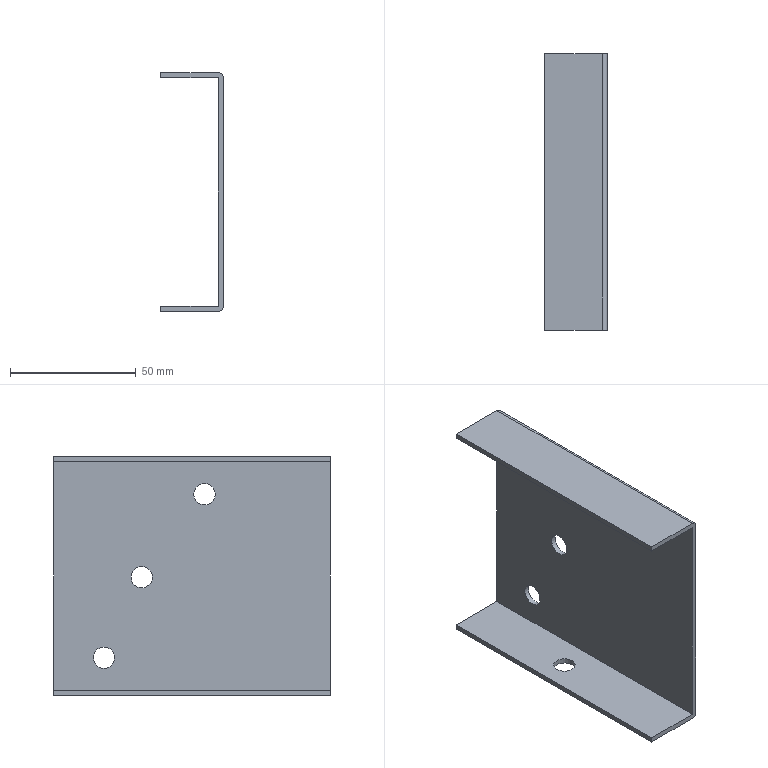Part | STEP file | 7470108L | 1 solid | 16 faces | box 25 x 110 x 95 mm | volume 30377 mm3 | plane 10 | cylinder 6 | commonest cylinder face diameters 8.5 x4 4 x2
STEP:
#1=CARTESIAN_POINT('',(0.,0.,0.));
#2=DIRECTION('',(0.,0.,1.));
#3=DIRECTION('',(1.,0.,0.));
#4=AXIS2_PLACEMENT_3D('',#1,#2,#3);
#5=CARTESIAN_POINT('',(-41.481,0.,45.198));
#6=VERTEX_POINT('',#5);
#7=CARTESIAN_POINT('',(-41.481,0.,43.198));
#8=VERTEX_POINT('',#7);
#9=CARTESIAN_POINT('',(-41.481,0.,43.198));
#10=DIRECTION('',(0.,0.,-1.));
#11=VECTOR('',#10,1.);
#12=LINE('',#9,#11);
#13=CARTESIAN_POINT('',(-41.481,110.,43.198));
#14=DIRECTION('',(1.,0.,0.));
#15=DIRECTION('',(0.,0.,1.));
#16=AXIS2_PLACEMENT_3D('',#13,#14,#15);
#17=PLANE('',#16);
#18=CARTESIAN_POINT('',(0.,110.));
#19=DIRECTION('',(-1.,0.));
#20=VECTOR('',#19,1.);
#21=LINE('',#18,#20);
#22=(GEOMETRIC_REPRESENTATION_CONTEXT(2)PARAMETRIC_REPRESENTATION_CONTEXT()REPRESENTATION_CONTEXT('',''));
#23=DEFINITIONAL_REPRESENTATION('',(#21),#22);
#24=PCURVE('',#17,#23);
#25=CARTESIAN_POINT('',(-18.481,0.,43.198));
#26=DIRECTION('',(0.,1.,0.));
#27=DIRECTION('',(0.,0.,1.));
#28=AXIS2_PLACEMENT_3D('',#25,#26,#27);
#29=PLANE('',#28);
#30=CARTESIAN_POINT('',(0.,-23.));
#31=DIRECTION('',(-1.,0.));
#32=VECTOR('',#31,1.);
#33=LINE('',#30,#32);
#34=(GEOMETRIC_REPRESENTATION_CONTEXT(2)PARAMETRIC_REPRESENTATION_CONTEXT()REPRESENTATION_CONTEXT('',''));
#35=DEFINITIONAL_REPRESENTATION('',(#33),#34);
#36=PCURVE('',#29,#35);
#37=SURFACE_CURVE('',#12,(#24,#36),.PCURVE_S1.);
#38=EDGE_CURVE('',#6,#8,#37,.T.);
#39=ORIENTED_EDGE('',*,*,#38,.F.);
#40=CARTESIAN_POINT('',(-41.481,110.,45.198));
#41=VERTEX_POINT('',#40);
#42=CARTESIAN_POINT('',(-41.481,110.,45.198));
#43=DIRECTION('',(0.,-1.,0.));
#44=VECTOR('',#43,1.);
#45=LINE('',#42,#44);
#46=CARTESIAN_POINT('',(2.,0.));
#47=DIRECTION('',(0.,1.));
#48=VECTOR('',#47,1.);
#49=LINE('',#46,#48);
#50=(GEOMETRIC_REPRESENTATION_CONTEXT(2)PARAMETRIC_REPRESENTATION_CONTEXT()REPRESENTATION_CONTEXT('',''));
#51=DEFINITIONAL_REPRESENTATION('',(#49),#50);
#52=PCURVE('',#17,#51);
#53=CARTESIAN_POINT('',(-18.481,110.,45.198));
#54=DIRECTION('',(0.,0.,-1.));
#55=DIRECTION('',(1.,0.,0.));
#56=AXIS2_PLACEMENT_3D('',#53,#54,#55);
#57=PLANE('',#56);
#58=CARTESIAN_POINT('',(-23.,0.));
#59=DIRECTION('',(0.,1.));
#60=VECTOR('',#59,1.);
#61=LINE('',#58,#60);
#62=(GEOMETRIC_REPRESENTATION_CONTEXT(2)PARAMETRIC_REPRESENTATION_CONTEXT()REPRESENTATION_CONTEXT('',''));
#63=DEFINITIONAL_REPRESENTATION('',(#61),#62);
#64=PCURVE('',#57,#63);
#65=SURFACE_CURVE('',#45,(#52,#64),.PCURVE_S1.);
#66=EDGE_CURVE('',#41,#6,#65,.T.);
#67=ORIENTED_EDGE('',*,*,#66,.F.);
#68=CARTESIAN_POINT('',(-41.481,110.,43.198));
#69=VERTEX_POINT('',#68);
#70=CARTESIAN_POINT('',(-41.481,110.,43.198));
#71=DIRECTION('',(0.,0.,-1.));
#72=VECTOR('',#71,1.);
#73=LINE('',#70,#72);
#74=CARTESIAN_POINT('',(0.,0.));
#75=DIRECTION('',(-1.,0.));
#76=VECTOR('',#75,1.);
#77=LINE('',#74,#76);
#78=(GEOMETRIC_REPRESENTATION_CONTEXT(2)PARAMETRIC_REPRESENTATION_CONTEXT()REPRESENTATION_CONTEXT('',''));
#79=DEFINITIONAL_REPRESENTATION('',(#77),#78);
#80=PCURVE('',#17,#79);
#81=CARTESIAN_POINT('',(-18.481,110.,43.198));
#82=DIRECTION('',(0.,1.,0.));
#83=DIRECTION('',(0.,0.,1.));
#84=AXIS2_PLACEMENT_3D('',#81,#82,#83);
#85=PLANE('',#84);
#86=CARTESIAN_POINT('',(0.,-23.));
#87=DIRECTION('',(-1.,0.));
#88=VECTOR('',#87,1.);
#89=LINE('',#86,#88);
#90=(GEOMETRIC_REPRESENTATION_CONTEXT(2)PARAMETRIC_REPRESENTATION_CONTEXT()REPRESENTATION_CONTEXT('',''));
#91=DEFINITIONAL_REPRESENTATION('',(#89),#90);
#92=PCURVE('',#85,#91);
#93=SURFACE_CURVE('',#73,(#80,#92),.PCURVE_S1.);
#94=EDGE_CURVE('',#41,#69,#93,.T.);
#95=ORIENTED_EDGE('',*,*,#94,.T.);
#96=CARTESIAN_POINT('',(-41.481,110.,43.198));
#97=DIRECTION('',(0.,-1.,0.));
#98=VECTOR('',#97,1.);
#99=LINE('',#96,#98);
#100=CARTESIAN_POINT('',(0.,0.));
#101=DIRECTION('',(0.,1.));
#102=VECTOR('',#101,1.);
#103=LINE('',#100,#102);
#104=(GEOMETRIC_REPRESENTATION_CONTEXT(2)PARAMETRIC_REPRESENTATION_CONTEXT()REPRESENTATION_CONTEXT('',''));
#105=DEFINITIONAL_REPRESENTATION('',(#103),#104);
#106=PCURVE('',#17,#105);
#107=CARTESIAN_POINT('',(-18.481,110.,43.198));
#108=DIRECTION('',(0.,0.,1.));
#109=DIRECTION('',(-1.,0.,0.));
#110=AXIS2_PLACEMENT_3D('',#107,#108,#109);
#111=PLANE('',#110);
#112=CARTESIAN_POINT('',(23.,0.));
#113=DIRECTION('',(0.,1.));
#114=VECTOR('',#113,1.);
#115=LINE('',#112,#114);
#116=(GEOMETRIC_REPRESENTATION_CONTEXT(2)PARAMETRIC_REPRESENTATION_CONTEXT()REPRESENTATION_CONTEXT('',''));
#117=DEFINITIONAL_REPRESENTATION('',(#115),#116);
#118=PCURVE('',#111,#117);
#119=SURFACE_CURVE('',#99,(#106,#118),.PCURVE_S1.);
#120=EDGE_CURVE('',#69,#8,#119,.T.);
#121=ORIENTED_EDGE('',*,*,#120,.T.);
#122=EDGE_LOOP('',(#39,#67,#95,#121));
#123=FACE_BOUND('',#122,.T.);
#124=ADVANCED_FACE('',(#123),#17,.F.);
#125=CARTESIAN_POINT('',(-18.481,0.,43.198));
#126=VERTEX_POINT('',#125);
#127=CARTESIAN_POINT('',(-18.481,0.,43.198));
#128=DIRECTION('',(1.,0.,0.));
#129=VECTOR('',#128,1.);
#130=LINE('',#127,#129);
#131=CARTESIAN_POINT('',(0.,110.));
#132=DIRECTION('',(-1.,0.));
#133=VECTOR('',#132,1.);
#134=LINE('',#131,#133);
#135=(GEOMETRIC_REPRESENTATION_CONTEXT(2)PARAMETRIC_REPRESENTATION_CONTEXT()REPRESENTATION_CONTEXT('',''));
#136=DEFINITIONAL_REPRESENTATION('',(#134),#135);
#137=PCURVE('',#111,#136);
#138=CARTESIAN_POINT('',(0.,0.));
#139=DIRECTION('',(0.,1.));
#140=VECTOR('',#139,1.);
#141=LINE('',#138,#140);
#142=(GEOMETRIC_REPRESENTATION_CONTEXT(2)PARAMETRIC_REPRESENTATION_CONTEXT()REPRESENTATION_CONTEXT('',''));
#143=DEFINITIONAL_REPRESENTATION('',(#141),#142);
#144=PCURVE('',#29,#143);
#145=SURFACE_CURVE('',#130,(#137,#144),.PCURVE_S1.);
#146=EDGE_CURVE('',#8,#126,#145,.T.);
#147=ORIENTED_EDGE('',*,*,#146,.F.);
#148=ORIENTED_EDGE('',*,*,#120,.F.);
#149=CARTESIAN_POINT('',(-18.481,110.,43.198));
#150=VERTEX_POINT('',#149);
#151=CARTESIAN_POINT('',(-18.481,110.,43.198));
#152=DIRECTION('',(1.,0.,0.));
#153=VECTOR('',#152,1.);
#154=LINE('',#151,#153);
#155=CARTESIAN_POINT('',(0.,0.));
#156=DIRECTION('',(-1.,0.));
#157=VECTOR('',#156,1.);
#158=LINE('',#155,#157);
#159=(GEOMETRIC_REPRESENTATION_CONTEXT(2)PARAMETRIC_REPRESENTATION_CONTEXT()REPRESENTATION_CONTEXT('',''));
#160=DEFINITIONAL_REPRESENTATION('',(#158),#159);
#161=PCURVE('',#111,#160);
#162=CARTESIAN_POINT('',(0.,0.));
#163=DIRECTION('',(0.,1.));
#164=VECTOR('',#163,1.);
#165=LINE('',#162,#164);
#166=(GEOMETRIC_REPRESENTATION_CONTEXT(2)PARAMETRIC_REPRESENTATION_CONTEXT()REPRESENTATION_CONTEXT('',''));
#167=DEFINITIONAL_REPRESENTATION('',(#165),#166);
#168=PCURVE('',#85,#167);
#169=SURFACE_CURVE('',#154,(#161,#168),.PCURVE_S1.);
#170=EDGE_CURVE('',#69,#150,#169,.T.);
#171=ORIENTED_EDGE('',*,*,#170,.T.);
#172=CARTESIAN_POINT('',(-18.481,110.,43.198));
#173=DIRECTION('',(0.,-1.,0.));
#174=VECTOR('',#173,1.);
#175=LINE('',#172,#174);
#176=CARTESIAN_POINT('',(0.,0.));
#177=DIRECTION('',(0.,1.));
#178=VECTOR('',#177,1.);
#179=LINE('',#176,#178);
#180=(GEOMETRIC_REPRESENTATION_CONTEXT(2)PARAMETRIC_REPRESENTATION_CONTEXT()REPRESENTATION_CONTEXT('',''));
#181=DEFINITIONAL_REPRESENTATION('',(#179),#180);
#182=PCURVE('',#111,#181);
#183=CARTESIAN_POINT('',(-18.481,110.,-47.802));
#184=DIRECTION('',(1.,0.,0.));
#185=DIRECTION('',(0.,0.,1.));
#186=AXIS2_PLACEMENT_3D('',#183,#184,#185);
#187=PLANE('',#186);
#188=CARTESIAN_POINT('',(91.,0.));
#189=DIRECTION('',(0.,1.));
#190=VECTOR('',#189,1.);
#191=LINE('',#188,#190);
#192=(GEOMETRIC_REPRESENTATION_CONTEXT(2)PARAMETRIC_REPRESENTATION_CONTEXT()REPRESENTATION_CONTEXT('',''));
#193=DEFINITIONAL_REPRESENTATION('',(#191),#192);
#194=PCURVE('',#187,#193);
#195=SURFACE_CURVE('',#175,(#182,#194),.PCURVE_S1.);
#196=EDGE_CURVE('',#150,#126,#195,.T.);
#197=ORIENTED_EDGE('',*,*,#196,.T.);
#198=EDGE_LOOP('',(#147,#148,#171,#197));
#199=FACE_BOUND('',#198,.T.);
#200=ADVANCED_FACE('',(#199),#111,.F.);
#201=CARTESIAN_POINT('',(-18.481,75.,1.448));
#202=VERTEX_POINT('',#201);
#203=CARTESIAN_POINT('',(-18.481,75.,-2.802));
#204=DIRECTION('',(-1.,0.,0.));
#205=DIRECTION('',(0.,0.,1.));
#206=AXIS2_PLACEMENT_3D('',#203,#204,#205);
#207=CIRCLE('',#206,4.25);
#208=CARTESIAN_POINT('',(49.25,35.));
#209=CARTESIAN_POINT('',(49.25,27.639));
#210=CARTESIAN_POINT('',(42.875,31.319));
#211=CARTESIAN_POINT('',(36.5,35.));
#212=CARTESIAN_POINT('',(42.875,38.681));
#213=CARTESIAN_POINT('',(49.25,42.361));
#214=CARTESIAN_POINT('',(49.25,35.));
#215=(BOUNDED_CURVE()B_SPLINE_CURVE(2,(#208,#209,#210,#211,#212,#213,#214),.UNSPECIFIED.,.T.,.F.)B_SPLINE_CURVE_WITH_KNOTS((1,2,2,2,2,1),(-2.094,0.,2.094,4.189,6.283,8.378),.UNSPECIFIED.)CURVE()GEOMETRIC_REPRESENTATION_ITEM()RATIONAL_B_SPLINE_CURVE((1.,0.5,1.,0.5,1.,0.5,1.))REPRESENTATION_ITEM(''));
#216=(GEOMETRIC_REPRESENTATION_CONTEXT(2)PARAMETRIC_REPRESENTATION_CONTEXT()REPRESENTATION_CONTEXT('',''));
#217=DEFINITIONAL_REPRESENTATION('',(#215),#216);
#218=PCURVE('',#187,#217);
#219=CARTESIAN_POINT('',(-26.481,75.,-2.802));
#220=DIRECTION('',(1.,0.,0.));
#221=DIRECTION('',(0.,0.,1.));
#222=AXIS2_PLACEMENT_3D('',#219,#220,#221);
#223=CYLINDRICAL_SURFACE('',#222,4.25);
#224=CARTESIAN_POINT('',(6.283,8.));
#225=DIRECTION('',(-1.,0.));
#226=VECTOR('',#225,1.);
#227=LINE('',#224,#226);
#228=(GEOMETRIC_REPRESENTATION_CONTEXT(2)PARAMETRIC_REPRESENTATION_CONTEXT()REPRESENTATION_CONTEXT('',''));
#229=DEFINITIONAL_REPRESENTATION('',(#227),#228);
#230=PCURVE('',#223,#229);
#231=SURFACE_CURVE('',#207,(#218,#230),.PCURVE_S1.);
#232=EDGE_CURVE('',#202,#202,#231,.T.);
#233=ORIENTED_EDGE('',*,*,#232,.F.);
#234=EDGE_LOOP('',(#233));
#235=FACE_BOUND('',#234,.T.);
#236=CARTESIAN_POINT('',(-18.481,50.,25.948));
#237=VERTEX_POINT('',#236);
#238=CARTESIAN_POINT('',(-18.481,50.,30.198));
#239=DIRECTION('',(1.,0.,0.));
#240=DIRECTION('',(0.,0.,-1.));
#241=AXIS2_PLACEMENT_3D('',#238,#239,#240);
#242=CIRCLE('',#241,4.25);
#243=CARTESIAN_POINT('',(78.,60.));
#244=DIRECTION('',(-1.,0.));
#245=AXIS2_PLACEMENT_2D('',#243,#244);
#246=CIRCLE('',#245,4.25);
#247=(GEOMETRIC_REPRESENTATION_CONTEXT(2)PARAMETRIC_REPRESENTATION_CONTEXT()REPRESENTATION_CONTEXT('',''));
#248=DEFINITIONAL_REPRESENTATION('',(#246),#247);
#249=PCURVE('',#187,#248);
#250=CARTESIAN_POINT('',(-8.481,50.,30.198));
#251=DIRECTION('',(-1.,0.,0.));
#252=DIRECTION('',(0.,0.,-1.));
#253=AXIS2_PLACEMENT_3D('',#250,#251,#252);
#254=CYLINDRICAL_SURFACE('',#253,4.25);
#255=CARTESIAN_POINT('',(6.283,10.));
#256=DIRECTION('',(-1.,0.));
#257=VECTOR('',#256,1.);
#258=LINE('',#255,#257);
#259=(GEOMETRIC_REPRESENTATION_CONTEXT(2)PARAMETRIC_REPRESENTATION_CONTEXT()REPRESENTATION_CONTEXT('',''));
#260=DEFINITIONAL_REPRESENTATION('',(#258),#259);
#261=PCURVE('',#254,#260);
#262=SURFACE_CURVE('',#242,(#249,#261),.PCURVE_S1.);
#263=EDGE_CURVE('',#237,#237,#262,.T.);
#264=ORIENTED_EDGE('',*,*,#263,.T.);
#265=EDGE_LOOP('',(#264));
#266=FACE_BOUND('',#265,.T.);
#267=CARTESIAN_POINT('',(-18.481,90.,-39.052));
#268=VERTEX_POINT('',#267);
#269=CARTESIAN_POINT('',(-18.481,90.,-34.802));
#270=DIRECTION('',(1.,0.,0.));
#271=DIRECTION('',(0.,0.,-1.));
#272=AXIS2_PLACEMENT_3D('',#269,#270,#271);
#273=CIRCLE('',#272,4.25);
#274=CARTESIAN_POINT('',(13.,20.));
#275=DIRECTION('',(-1.,0.));
#276=AXIS2_PLACEMENT_2D('',#274,#275);
#277=CIRCLE('',#276,4.25);
#278=(GEOMETRIC_REPRESENTATION_CONTEXT(2)PARAMETRIC_REPRESENTATION_CONTEXT()REPRESENTATION_CONTEXT('',''));
#279=DEFINITIONAL_REPRESENTATION('',(#277),#278);
#280=PCURVE('',#187,#279);
#281=CARTESIAN_POINT('',(-8.481,90.,-34.802));
#282=DIRECTION('',(-1.,0.,0.));
#283=DIRECTION('',(0.,0.,-1.));
#284=AXIS2_PLACEMENT_3D('',#281,#282,#283);
#285=CYLINDRICAL_SURFACE('',#284,4.25);
#286=CARTESIAN_POINT('',(6.283,10.));
#287=DIRECTION('',(-1.,0.));
#288=VECTOR('',#287,1.);
#289=LINE('',#286,#288);
#290=(GEOMETRIC_REPRESENTATION_CONTEXT(2)PARAMETRIC_REPRESENTATION_CONTEXT()REPRESENTATION_CONTEXT('',''));
#291=DEFINITIONAL_REPRESENTATION('',(#289),#290);
#292=PCURVE('',#285,#291);
#293=SURFACE_CURVE('',#273,(#280,#292),.PCURVE_S1.);
#294=EDGE_CURVE('',#268,#268,#293,.T.);
#295=ORIENTED_EDGE('',*,*,#294,.T.);
#296=EDGE_LOOP('',(#295));
#297=FACE_BOUND('',#296,.T.);
#298=CARTESIAN_POINT('',(-18.481,0.,-47.802));
#299=VERTEX_POINT('',#298);
#300=CARTESIAN_POINT('',(-18.481,0.,-47.802));
#301=DIRECTION('',(0.,0.,-1.));
#302=VECTOR('',#301,1.);
#303=LINE('',#300,#302);
#304=CARTESIAN_POINT('',(0.,110.));
#305=DIRECTION('',(-1.,0.));
#306=VECTOR('',#305,1.);
#307=LINE('',#304,#306);
#308=(GEOMETRIC_REPRESENTATION_CONTEXT(2)PARAMETRIC_REPRESENTATION_CONTEXT()REPRESENTATION_CONTEXT('',''));
#309=DEFINITIONAL_REPRESENTATION('',(#307),#308);
#310=PCURVE('',#187,#309);
#311=CARTESIAN_POINT('',(-91.,0.));
#312=DIRECTION('',(-1.,0.));
#313=VECTOR('',#312,1.);
#314=LINE('',#311,#313);
#315=(GEOMETRIC_REPRESENTATION_CONTEXT(2)PARAMETRIC_REPRESENTATION_CONTEXT()REPRESENTATION_CONTEXT('',''));
#316=DEFINITIONAL_REPRESENTATION('',(#314),#315);
#317=PCURVE('',#29,#316);
#318=SURFACE_CURVE('',#303,(#310,#317),.PCURVE_S1.);
#319=EDGE_CURVE('',#126,#299,#318,.T.);
#320=ORIENTED_EDGE('',*,*,#319,.F.);
#321=ORIENTED_EDGE('',*,*,#196,.F.);
#322=CARTESIAN_POINT('',(-18.481,110.,-47.802));
#323=VERTEX_POINT('',#322);
#324=CARTESIAN_POINT('',(-18.481,110.,-47.802));
#325=DIRECTION('',(0.,0.,-1.));
#326=VECTOR('',#325,1.);
#327=LINE('',#324,#326);
#328=CARTESIAN_POINT('',(0.,0.));
#329=DIRECTION('',(-1.,0.));
#330=VECTOR('',#329,1.);
#331=LINE('',#328,#330);
#332=(GEOMETRIC_REPRESENTATION_CONTEXT(2)PARAMETRIC_REPRESENTATION_CONTEXT()REPRESENTATION_CONTEXT('',''));
#333=DEFINITIONAL_REPRESENTATION('',(#331),#332);
#334=PCURVE('',#187,#333);
#335=CARTESIAN_POINT('',(-91.,0.));
#336=DIRECTION('',(-1.,0.));
#337=VECTOR('',#336,1.);
#338=LINE('',#335,#337);
#339=(GEOMETRIC_REPRESENTATION_CONTEXT(2)PARAMETRIC_REPRESENTATION_CONTEXT()REPRESENTATION_CONTEXT('',''));
#340=DEFINITIONAL_REPRESENTATION('',(#338),#339);
#341=PCURVE('',#85,#340);
#342=SURFACE_CURVE('',#327,(#334,#341),.PCURVE_S1.);
#343=EDGE_CURVE('',#150,#323,#342,.T.);
#344=ORIENTED_EDGE('',*,*,#343,.T.);
#345=CARTESIAN_POINT('',(-18.481,110.,-47.802));
#346=DIRECTION('',(0.,-1.,0.));
#347=VECTOR('',#346,1.);
#348=LINE('',#345,#347);
#349=CARTESIAN_POINT('',(0.,0.));
#350=DIRECTION('',(0.,1.));
#351=VECTOR('',#350,1.);
#352=LINE('',#349,#351);
#353=(GEOMETRIC_REPRESENTATION_CONTEXT(2)PARAMETRIC_REPRESENTATION_CONTEXT()REPRESENTATION_CONTEXT('',''));
#354=DEFINITIONAL_REPRESENTATION('',(#352),#353);
#355=PCURVE('',#187,#354);
#356=CARTESIAN_POINT('',(-18.481,110.,-47.802));
#357=DIRECTION('',(0.,0.,-1.));
#358=DIRECTION('',(1.,0.,0.));
#359=AXIS2_PLACEMENT_3D('',#356,#357,#358);
#360=PLANE('',#359);
#361=CARTESIAN_POINT('',(0.,0.));
#362=DIRECTION('',(0.,1.));
#363=VECTOR('',#362,1.);
#364=LINE('',#361,#363);
#365=(GEOMETRIC_REPRESENTATION_CONTEXT(2)PARAMETRIC_REPRESENTATION_CONTEXT()REPRESENTATION_CONTEXT('',''));
#366=DEFINITIONAL_REPRESENTATION('',(#364),#365);
#367=PCURVE('',#360,#366);
#368=SURFACE_CURVE('',#348,(#355,#367),.PCURVE_S1.);
#369=EDGE_CURVE('',#323,#299,#368,.T.);
#370=ORIENTED_EDGE('',*,*,#369,.T.);
#371=EDGE_LOOP('',(#320,#321,#344,#370));
#372=FACE_BOUND('',#371,.T.);
#373=ADVANCED_FACE('',(#235,#266,#297,#372),#187,.F.);
#374=CARTESIAN_POINT('',(-26.231,60.,-47.802));
#375=VERTEX_POINT('',#374);
#376=CARTESIAN_POINT('',(-30.481,60.,-47.802));
#377=DIRECTION('',(0.,0.,1.));
#378=DIRECTION('',(1.,0.,0.));
#379=AXIS2_PLACEMENT_3D('',#376,#377,#378);
#380=CIRCLE('',#379,4.25);
#381=CARTESIAN_POINT('',(-7.75,50.));
#382=CARTESIAN_POINT('',(-7.75,42.639));
#383=CARTESIAN_POINT('',(-14.125,46.319));
#384=CARTESIAN_POINT('',(-20.5,50.));
#385=CARTESIAN_POINT('',(-14.125,53.681));
#386=CARTESIAN_POINT('',(-7.75,57.361));
#387=CARTESIAN_POINT('',(-7.75,50.));
#388=(BOUNDED_CURVE()B_SPLINE_CURVE(2,(#381,#382,#383,#384,#385,#386,#387),.UNSPECIFIED.,.T.,.F.)B_SPLINE_CURVE_WITH_KNOTS((1,2,2,2,2,1),(-2.094,0.,2.094,4.189,6.283,8.378),.UNSPECIFIED.)CURVE()GEOMETRIC_REPRESENTATION_ITEM()RATIONAL_B_SPLINE_CURVE((1.,0.5,1.,0.5,1.,0.5,1.))REPRESENTATION_ITEM(''));
#389=(GEOMETRIC_REPRESENTATION_CONTEXT(2)PARAMETRIC_REPRESENTATION_CONTEXT()REPRESENTATION_CONTEXT('',''));
#390=DEFINITIONAL_REPRESENTATION('',(#388),#389);
#391=PCURVE('',#360,#390);
#392=CARTESIAN_POINT('',(-30.481,60.,-39.802));
#393=DIRECTION('',(0.,0.,-1.));
#394=DIRECTION('',(1.,0.,0.));
#395=AXIS2_PLACEMENT_3D('',#392,#393,#394);
#396=CYLINDRICAL_SURFACE('',#395,4.25);
#397=CARTESIAN_POINT('',(6.283,8.));
#398=DIRECTION('',(-1.,0.));
#399=VECTOR('',#398,1.);
#400=LINE('',#397,#399);
#401=(GEOMETRIC_REPRESENTATION_CONTEXT(2)PARAMETRIC_REPRESENTATION_CONTEXT()REPRESENTATION_CONTEXT('',''));
#402=DEFINITIONAL_REPRESENTATION('',(#400),#401);
#403=PCURVE('',#396,#402);
#404=SURFACE_CURVE('',#380,(#391,#403),.PCURVE_S1.);
#405=EDGE_CURVE('',#375,#375,#404,.T.);
#406=ORIENTED_EDGE('',*,*,#405,.F.);
#407=EDGE_LOOP('',(#406));
#408=FACE_BOUND('',#407,.T.);
#409=CARTESIAN_POINT('',(-41.481,0.,-47.802));
#410=VERTEX_POINT('',#409);
#411=CARTESIAN_POINT('',(-18.481,0.,-47.802));
#412=DIRECTION('',(-1.,0.,0.));
#413=VECTOR('',#412,1.);
#414=LINE('',#411,#413);
#415=CARTESIAN_POINT('',(0.,110.));
#416=DIRECTION('',(-1.,0.));
#417=VECTOR('',#416,1.);
#418=LINE('',#415,#417);
#419=(GEOMETRIC_REPRESENTATION_CONTEXT(2)PARAMETRIC_REPRESENTATION_CONTEXT()REPRESENTATION_CONTEXT('',''));
#420=DEFINITIONAL_REPRESENTATION('',(#418),#419);
#421=PCURVE('',#360,#420);
#422=CARTESIAN_POINT('',(-91.,0.));
#423=DIRECTION('',(0.,-1.));
#424=VECTOR('',#423,1.);
#425=LINE('',#422,#424);
#426=(GEOMETRIC_REPRESENTATION_CONTEXT(2)PARAMETRIC_REPRESENTATION_CONTEXT()REPRESENTATION_CONTEXT('',''));
#427=DEFINITIONAL_REPRESENTATION('',(#425),#426);
#428=PCURVE('',#29,#427);
#429=SURFACE_CURVE('',#414,(#421,#428),.PCURVE_S1.);
#430=EDGE_CURVE('',#299,#410,#429,.T.);
#431=ORIENTED_EDGE('',*,*,#430,.F.);
#432=ORIENTED_EDGE('',*,*,#369,.F.);
#433=CARTESIAN_POINT('',(-41.481,110.,-47.802));
#434=VERTEX_POINT('',#433);
#435=CARTESIAN_POINT('',(-18.481,110.,-47.802));
#436=DIRECTION('',(-1.,0.,0.));
#437=VECTOR('',#436,1.);
#438=LINE('',#435,#437);
#439=CARTESIAN_POINT('',(0.,0.));
#440=DIRECTION('',(-1.,0.));
#441=VECTOR('',#440,1.);
#442=LINE('',#439,#441);
#443=(GEOMETRIC_REPRESENTATION_CONTEXT(2)PARAMETRIC_REPRESENTATION_CONTEXT()REPRESENTATION_CONTEXT('',''));
#444=DEFINITIONAL_REPRESENTATION('',(#442),#443);
#445=PCURVE('',#360,#444);
#446=CARTESIAN_POINT('',(-91.,0.));
#447=DIRECTION('',(0.,-1.));
#448=VECTOR('',#447,1.);
#449=LINE('',#446,#448);
#450=(GEOMETRIC_REPRESENTATION_CONTEXT(2)PARAMETRIC_REPRESENTATION_CONTEXT()REPRESENTATION_CONTEXT('',''));
#451=DEFINITIONAL_REPRESENTATION('',(#449),#450);
#452=PCURVE('',#85,#451);
#453=SURFACE_CURVE('',#438,(#445,#452),.PCURVE_S1.);
#454=EDGE_CURVE('',#323,#434,#453,.T.);
#455=ORIENTED_EDGE('',*,*,#454,.T.);
#456=CARTESIAN_POINT('',(-41.481,110.,-47.802));
#457=DIRECTION('',(0.,-1.,0.));
#458=VECTOR('',#457,1.);
#459=LINE('',#456,#458);
#460=CARTESIAN_POINT('',(-23.,0.));
#461=DIRECTION('',(0.,1.));
#462=VECTOR('',#461,1.);
#463=LINE('',#460,#462);
#464=(GEOMETRIC_REPRESENTATION_CONTEXT(2)PARAMETRIC_REPRESENTATION_CONTEXT()REPRESENTATION_CONTEXT('',''));
#465=DEFINITIONAL_REPRESENTATION('',(#463),#464);
#466=PCURVE('',#360,#465);
#467=CARTESIAN_POINT('',(-41.481,110.,-49.802));
#468=DIRECTION('',(1.,0.,0.));
#469=DIRECTION('',(0.,0.,1.));
#470=AXIS2_PLACEMENT_3D('',#467,#468,#469);
#471=PLANE('',#470);
#472=CARTESIAN_POINT('',(2.,0.));
#473=DIRECTION('',(0.,1.));
#474=VECTOR('',#473,1.);
#475=LINE('',#472,#474);
#476=(GEOMETRIC_REPRESENTATION_CONTEXT(2)PARAMETRIC_REPRESENTATION_CONTEXT()REPRESENTATION_CONTEXT('',''));
#477=DEFINITIONAL_REPRESENTATION('',(#475),#476);
#478=PCURVE('',#471,#477);
#479=SURFACE_CURVE('',#459,(#466,#478),.PCURVE_S1.);
#480=EDGE_CURVE('',#434,#410,#479,.T.);
#481=ORIENTED_EDGE('',*,*,#480,.T.);
#482=EDGE_LOOP('',(#431,#432,#455,#481));
#483=FACE_BOUND('',#482,.T.);
#484=ADVANCED_FACE('',(#408,#483),#360,.F.);
#485=CARTESIAN_POINT('',(-41.481,0.,-49.802));
#486=VERTEX_POINT('',#485);
#487=CARTESIAN_POINT('',(-41.481,0.,-49.802));
#488=DIRECTION('',(0.,0.,-1.));
#489=VECTOR('',#488,1.);
#490=LINE('',#487,#489);
#491=CARTESIAN_POINT('',(0.,110.));
#492=DIRECTION('',(-1.,0.));
#493=VECTOR('',#492,1.);
#494=LINE('',#491,#493);
#495=(GEOMETRIC_REPRESENTATION_CONTEXT(2)PARAMETRIC_REPRESENTATION_CONTEXT()REPRESENTATION_CONTEXT('',''));
#496=DEFINITIONAL_REPRESENTATION('',(#494),#495);
#497=PCURVE('',#471,#496);
#498=CARTESIAN_POINT('',(-93.,-23.));
#499=DIRECTION('',(-1.,0.));
#500=VECTOR('',#499,1.);
#501=LINE('',#498,#500);
#502=(GEOMETRIC_REPRESENTATION_CONTEXT(2)PARAMETRIC_REPRESENTATION_CONTEXT()REPRESENTATION_CONTEXT('',''));
#503=DEFINITIONAL_REPRESENTATION('',(#501),#502);
#504=PCURVE('',#29,#503);
#505=SURFACE_CURVE('',#490,(#497,#504),.PCURVE_S1.);
#506=EDGE_CURVE('',#410,#486,#505,.T.);
#507=ORIENTED_EDGE('',*,*,#506,.F.);
#508=ORIENTED_EDGE('',*,*,#480,.F.);
#509=CARTESIAN_POINT('',(-41.481,110.,-49.802));
#510=VERTEX_POINT('',#509);
#511=CARTESIAN_POINT('',(-41.481,110.,-49.802));
#512=DIRECTION('',(0.,0.,-1.));
#513=VECTOR('',#512,1.);
#514=LINE('',#511,#513);
#515=CARTESIAN_POINT('',(0.,0.));
#516=DIRECTION('',(-1.,0.));
#517=VECTOR('',#516,1.);
#518=LINE('',#515,#517);
#519=(GEOMETRIC_REPRESENTATION_CONTEXT(2)PARAMETRIC_REPRESENTATION_CONTEXT()REPRESENTATION_CONTEXT('',''));
#520=DEFINITIONAL_REPRESENTATION('',(#518),#519);
#521=PCURVE('',#471,#520);
#522=CARTESIAN_POINT('',(-93.,-23.));
#523=DIRECTION('',(-1.,0.));
#524=VECTOR('',#523,1.);
#525=LINE('',#522,#524);
#526=(GEOMETRIC_REPRESENTATION_CONTEXT(2)PARAMETRIC_REPRESENTATION_CONTEXT()REPRESENTATION_CONTEXT('',''));
#527=DEFINITIONAL_REPRESENTATION('',(#525),#526);
#528=PCURVE('',#85,#527);
#529=SURFACE_CURVE('',#514,(#521,#528),.PCURVE_S1.);
#530=EDGE_CURVE('',#434,#510,#529,.T.);
#531=ORIENTED_EDGE('',*,*,#530,.T.);
#532=CARTESIAN_POINT('',(-41.481,110.,-49.802));
#533=DIRECTION('',(0.,-1.,0.));
#534=VECTOR('',#533,1.);
#535=LINE('',#532,#534);
#536=CARTESIAN_POINT('',(0.,0.));
#537=DIRECTION('',(0.,1.));
#538=VECTOR('',#537,1.);
#539=LINE('',#536,#538);
#540=(GEOMETRIC_REPRESENTATION_CONTEXT(2)PARAMETRIC_REPRESENTATION_CONTEXT()REPRESENTATION_CONTEXT('',''));
#541=DEFINITIONAL_REPRESENTATION('',(#539),#540);
#542=PCURVE('',#471,#541);
#543=CARTESIAN_POINT('',(-18.481,110.,-49.802));
#544=DIRECTION('',(0.,0.,1.));
#545=DIRECTION('',(-1.,0.,0.));
#546=AXIS2_PLACEMENT_3D('',#543,#544,#545);
#547=PLANE('',#546);
#548=CARTESIAN_POINT('',(23.,0.));
#549=DIRECTION('',(0.,1.));
#550=VECTOR('',#549,1.);
#551=LINE('',#548,#550);
#552=(GEOMETRIC_REPRESENTATION_CONTEXT(2)PARAMETRIC_REPRESENTATION_CONTEXT()REPRESENTATION_CONTEXT('',''));
#553=DEFINITIONAL_REPRESENTATION('',(#551),#552);
#554=PCURVE('',#547,#553);
#555=SURFACE_CURVE('',#535,(#542,#554),.PCURVE_S1.);
#556=EDGE_CURVE('',#510,#486,#555,.T.);
#557=ORIENTED_EDGE('',*,*,#556,.T.);
#558=EDGE_LOOP('',(#507,#508,#531,#557));
#559=FACE_BOUND('',#558,.T.);
#560=ADVANCED_FACE('',(#559),#471,.F.);
#561=CARTESIAN_POINT('',(-26.231,60.,-49.802));
#562=VERTEX_POINT('',#561);
#563=CARTESIAN_POINT('',(-30.481,60.,-49.802));
#564=DIRECTION('',(0.,0.,1.));
#565=DIRECTION('',(1.,0.,0.));
#566=AXIS2_PLACEMENT_3D('',#563,#564,#565);
#567=CIRCLE('',#566,4.25);
#568=CARTESIAN_POINT('',(12.,50.));
#569=DIRECTION('',(-1.,0.));
#570=AXIS2_PLACEMENT_2D('',#568,#569);
#571=CIRCLE('',#570,4.25);
#572=(GEOMETRIC_REPRESENTATION_CONTEXT(2)PARAMETRIC_REPRESENTATION_CONTEXT()REPRESENTATION_CONTEXT('',''));
#573=DEFINITIONAL_REPRESENTATION('',(#571),#572);
#574=PCURVE('',#547,#573);
#575=CARTESIAN_POINT('',(6.283,10.));
#576=DIRECTION('',(-1.,0.));
#577=VECTOR('',#576,1.);
#578=LINE('',#575,#577);
#579=(GEOMETRIC_REPRESENTATION_CONTEXT(2)PARAMETRIC_REPRESENTATION_CONTEXT()REPRESENTATION_CONTEXT('',''));
#580=DEFINITIONAL_REPRESENTATION('',(#578),#579);
#581=PCURVE('',#396,#580);
#582=SURFACE_CURVE('',#567,(#574,#581),.PCURVE_S1.);
#583=EDGE_CURVE('',#562,#562,#582,.T.);
#584=ORIENTED_EDGE('',*,*,#583,.T.);
#585=EDGE_LOOP('',(#584));
#586=FACE_BOUND('',#585,.T.);
#587=CARTESIAN_POINT('',(-18.481,0.,-49.802));
#588=VERTEX_POINT('',#587);
#589=CARTESIAN_POINT('',(-18.481,0.,-49.802));
#590=DIRECTION('',(1.,0.,0.));
#591=VECTOR('',#590,1.);
#592=LINE('',#589,#591);
#593=CARTESIAN_POINT('',(0.,110.));
#594=DIRECTION('',(-1.,0.));
#595=VECTOR('',#594,1.);
#596=LINE('',#593,#595);
#597=(GEOMETRIC_REPRESENTATION_CONTEXT(2)PARAMETRIC_REPRESENTATION_CONTEXT()REPRESENTATION_CONTEXT('',''));
#598=DEFINITIONAL_REPRESENTATION('',(#596),#597);
#599=PCURVE('',#547,#598);
#600=CARTESIAN_POINT('',(-93.,0.));
#601=DIRECTION('',(0.,1.));
#602=VECTOR('',#601,1.);
#603=LINE('',#600,#602);
#604=(GEOMETRIC_REPRESENTATION_CONTEXT(2)PARAMETRIC_REPRESENTATION_CONTEXT()REPRESENTATION_CONTEXT('',''));
#605=DEFINITIONAL_REPRESENTATION('',(#603),#604);
#606=PCURVE('',#29,#605);
#607=SURFACE_CURVE('',#592,(#599,#606),.PCURVE_S1.);
#608=EDGE_CURVE('',#486,#588,#607,.T.);
#609=ORIENTED_EDGE('',*,*,#608,.F.);
#610=ORIENTED_EDGE('',*,*,#556,.F.);
#611=CARTESIAN_POINT('',(-18.481,110.,-49.802));
#612=VERTEX_POINT('',#611);
#613=CARTESIAN_POINT('',(-18.481,110.,-49.802));
#614=DIRECTION('',(1.,0.,0.));
#615=VECTOR('',#614,1.);
#616=LINE('',#613,#615);
#617=CARTESIAN_POINT('',(0.,0.));
#618=DIRECTION('',(-1.,0.));
#619=VECTOR('',#618,1.);
#620=LINE('',#617,#619);
#621=(GEOMETRIC_REPRESENTATION_CONTEXT(2)PARAMETRIC_REPRESENTATION_CONTEXT()REPRESENTATION_CONTEXT('',''));
#622=DEFINITIONAL_REPRESENTATION('',(#620),#621);
#623=PCURVE('',#547,#622);
#624=CARTESIAN_POINT('',(-93.,0.));
#625=DIRECTION('',(0.,1.));
#626=VECTOR('',#625,1.);
#627=LINE('',#624,#626);
#628=(GEOMETRIC_REPRESENTATION_CONTEXT(2)PARAMETRIC_REPRESENTATION_CONTEXT()REPRESENTATION_CONTEXT('',''));
#629=DEFINITIONAL_REPRESENTATION('',(#627),#628);
#630=PCURVE('',#85,#629);
#631=SURFACE_CURVE('',#616,(#623,#630),.PCURVE_S1.);
#632=EDGE_CURVE('',#510,#612,#631,.T.);
#633=ORIENTED_EDGE('',*,*,#632,.T.);
#634=CARTESIAN_POINT('',(-18.481,110.,-49.802));
#635=DIRECTION('',(0.,-1.,0.));
#636=VECTOR('',#635,1.);
#637=LINE('',#634,#636);
#638=CARTESIAN_POINT('',(0.,0.));
#639=DIRECTION('',(0.,1.));
#640=VECTOR('',#639,1.);
#641=LINE('',#638,#640);
#642=(GEOMETRIC_REPRESENTATION_CONTEXT(2)PARAMETRIC_REPRESENTATION_CONTEXT()REPRESENTATION_CONTEXT('',''));
#643=DEFINITIONAL_REPRESENTATION('',(#641),#642);
#644=PCURVE('',#547,#643);
#645=CARTESIAN_POINT('',(-18.481,110.,-47.802));
#646=DIRECTION('',(0.,-1.,0.));
#647=DIRECTION('',(0.,0.,-1.));
#648=AXIS2_PLACEMENT_3D('',#645,#646,#647);
#649=CYLINDRICAL_SURFACE('',#648,2.);
#650=CARTESIAN_POINT('',(0.,0.));
#651=DIRECTION('',(0.,1.));
#652=VECTOR('',#651,1.);
#653=LINE('',#650,#652);
#654=(GEOMETRIC_REPRESENTATION_CONTEXT(2)PARAMETRIC_REPRESENTATION_CONTEXT()REPRESENTATION_CONTEXT('',''));
#655=DEFINITIONAL_REPRESENTATION('',(#653),#654);
#656=PCURVE('',#649,#655);
#657=SURFACE_CURVE('',#637,(#644,#656),.PCURVE_S1.);
#658=EDGE_CURVE('',#612,#588,#657,.T.);
#659=ORIENTED_EDGE('',*,*,#658,.T.);
#660=EDGE_LOOP('',(#609,#610,#633,#659));
#661=FACE_BOUND('',#660,.T.);
#662=ADVANCED_FACE('',(#586,#661),#547,.F.);
#663=CARTESIAN_POINT('',(-16.481,0.,-47.802));
#664=VERTEX_POINT('',#663);
#665=CARTESIAN_POINT('',(-18.481,0.,-47.802));
#666=DIRECTION('',(0.,-1.,0.));
#667=DIRECTION('',(0.,0.,-1.));
#668=AXIS2_PLACEMENT_3D('',#665,#666,#667);
#669=CIRCLE('',#668,2.);
#670=CARTESIAN_POINT('',(0.,110.));
#671=DIRECTION('',(1.,0.));
#672=VECTOR('',#671,1.);
#673=LINE('',#670,#672);
#674=(GEOMETRIC_REPRESENTATION_CONTEXT(2)PARAMETRIC_REPRESENTATION_CONTEXT()REPRESENTATION_CONTEXT('',''));
#675=DEFINITIONAL_REPRESENTATION('',(#673),#674);
#676=PCURVE('',#649,#675);
#677=CARTESIAN_POINT('',(-93.,0.));
#678=CARTESIAN_POINT('',(-93.,3.464));
#679=CARTESIAN_POINT('',(-90.,1.732));
#680=CARTESIAN_POINT('',(-87.,0.));
#681=CARTESIAN_POINT('',(-90.,-1.732));
#682=CARTESIAN_POINT('',(-93.,-3.464));
#683=CARTESIAN_POINT('',(-93.,0.));
#684=(BOUNDED_CURVE()B_SPLINE_CURVE(2,(#677,#678,#679,#680,#681,#682,#683),.UNSPECIFIED.,.T.,.F.)B_SPLINE_CURVE_WITH_KNOTS((1,2,2,2,2,1),(-2.094,0.,2.094,4.189,6.283,8.378),.UNSPECIFIED.)CURVE()GEOMETRIC_REPRESENTATION_ITEM()RATIONAL_B_SPLINE_CURVE((1.,0.5,1.,0.5,1.,0.5,1.))REPRESENTATION_ITEM(''));
#685=(GEOMETRIC_REPRESENTATION_CONTEXT(2)PARAMETRIC_REPRESENTATION_CONTEXT()REPRESENTATION_CONTEXT('',''));
#686=DEFINITIONAL_REPRESENTATION('',(#684),#685);
#687=PCURVE('',#29,#686);
#688=SURFACE_CURVE('',#669,(#676,#687),.PCURVE_S1.);
#689=EDGE_CURVE('',#588,#664,#688,.T.);
#690=ORIENTED_EDGE('',*,*,#689,.F.);
#691=ORIENTED_EDGE('',*,*,#658,.F.);
#692=CARTESIAN_POINT('',(-16.481,110.,-47.802));
#693=VERTEX_POINT('',#692);
#694=CARTESIAN_POINT('',(-18.481,110.,-47.802));
#695=DIRECTION('',(0.,-1.,0.));
#696=DIRECTION('',(0.,0.,-1.));
#697=AXIS2_PLACEMENT_3D('',#694,#695,#696);
#698=CIRCLE('',#697,2.);
#699=CARTESIAN_POINT('',(0.,0.));
#700=DIRECTION('',(1.,0.));
#701=VECTOR('',#700,1.);
#702=LINE('',#699,#701);
#703=(GEOMETRIC_REPRESENTATION_CONTEXT(2)PARAMETRIC_REPRESENTATION_CONTEXT()REPRESENTATION_CONTEXT('',''));
#704=DEFINITIONAL_REPRESENTATION('',(#702),#703);
#705=PCURVE('',#649,#704);
#706=CARTESIAN_POINT('',(-93.,0.));
#707=CARTESIAN_POINT('',(-93.,3.464));
#708=CARTESIAN_POINT('',(-90.,1.732));
#709=CARTESIAN_POINT('',(-87.,0.));
#710=CARTESIAN_POINT('',(-90.,-1.732));
#711=CARTESIAN_POINT('',(-93.,-3.464));
#712=CARTESIAN_POINT('',(-93.,0.));
#713=(BOUNDED_CURVE()B_SPLINE_CURVE(2,(#706,#707,#708,#709,#710,#711,#712),.UNSPECIFIED.,.T.,.F.)B_SPLINE_CURVE_WITH_KNOTS((1,2,2,2,2,1),(-2.094,0.,2.094,4.189,6.283,8.378),.UNSPECIFIED.)CURVE()GEOMETRIC_REPRESENTATION_ITEM()RATIONAL_B_SPLINE_CURVE((1.,0.5,1.,0.5,1.,0.5,1.))REPRESENTATION_ITEM(''));
#714=(GEOMETRIC_REPRESENTATION_CONTEXT(2)PARAMETRIC_REPRESENTATION_CONTEXT()REPRESENTATION_CONTEXT('',''));
#715=DEFINITIONAL_REPRESENTATION('',(#713),#714);
#716=PCURVE('',#85,#715);
#717=SURFACE_CURVE('',#698,(#705,#716),.PCURVE_S1.);
#718=EDGE_CURVE('',#612,#693,#717,.T.);
#719=ORIENTED_EDGE('',*,*,#718,.T.);
#720=CARTESIAN_POINT('',(-16.481,110.,-47.802));
#721=DIRECTION('',(0.,-1.,0.));
#722=VECTOR('',#721,1.);
#723=LINE('',#720,#722);
#724=CARTESIAN_POINT('',(1.571,0.));
#725=DIRECTION('',(0.,1.));
#726=VECTOR('',#725,1.);
#727=LINE('',#724,#726);
#728=(GEOMETRIC_REPRESENTATION_CONTEXT(2)PARAMETRIC_REPRESENTATION_CONTEXT()REPRESENTATION_CONTEXT('',''));
#729=DEFINITIONAL_REPRESENTATION('',(#727),#728);
#730=PCURVE('',#649,#729);
#731=CARTESIAN_POINT('',(-16.481,110.,-47.802));
#732=DIRECTION('',(-1.,0.,0.));
#733=DIRECTION('',(0.,0.,-1.));
#734=AXIS2_PLACEMENT_3D('',#731,#732,#733);
#735=PLANE('',#734);
#736=CARTESIAN_POINT('',(0.,0.));
#737=DIRECTION('',(0.,1.));
#738=VECTOR('',#737,1.);
#739=LINE('',#736,#738);
#740=(GEOMETRIC_REPRESENTATION_CONTEXT(2)PARAMETRIC_REPRESENTATION_CONTEXT()REPRESENTATION_CONTEXT('',''));
#741=DEFINITIONAL_REPRESENTATION('',(#739),#740);
#742=PCURVE('',#735,#741);
#743=SURFACE_CURVE('',#723,(#730,#742),.PCURVE_S1.);
#744=EDGE_CURVE('',#693,#664,#743,.T.);
#745=ORIENTED_EDGE('',*,*,#744,.T.);
#746=EDGE_LOOP('',(#690,#691,#719,#745));
#747=FACE_BOUND('',#746,.T.);
#748=ADVANCED_FACE('',(#747),#649,.T.);
#749=CARTESIAN_POINT('',(-16.481,75.,1.448));
#750=VERTEX_POINT('',#749);
#751=CARTESIAN_POINT('',(-16.481,75.,-2.802));
#752=DIRECTION('',(-1.,0.,0.));
#753=DIRECTION('',(0.,0.,1.));
#754=AXIS2_PLACEMENT_3D('',#751,#752,#753);
#755=CIRCLE('',#754,4.25);
#756=CARTESIAN_POINT('',(-45.,35.));
#757=DIRECTION('',(-1.,0.));
#758=AXIS2_PLACEMENT_2D('',#756,#757);
#759=CIRCLE('',#758,4.25);
#760=(GEOMETRIC_REPRESENTATION_CONTEXT(2)PARAMETRIC_REPRESENTATION_CONTEXT()REPRESENTATION_CONTEXT('',''));
#761=DEFINITIONAL_REPRESENTATION('',(#759),#760);
#762=PCURVE('',#735,#761);
#763=CARTESIAN_POINT('',(6.283,10.));
#764=DIRECTION('',(-1.,0.));
#765=VECTOR('',#764,1.);
#766=LINE('',#763,#765);
#767=(GEOMETRIC_REPRESENTATION_CONTEXT(2)PARAMETRIC_REPRESENTATION_CONTEXT()REPRESENTATION_CONTEXT('',''));
#768=DEFINITIONAL_REPRESENTATION('',(#766),#767);
#769=PCURVE('',#223,#768);
#770=SURFACE_CURVE('',#755,(#762,#769),.PCURVE_S1.);
#771=EDGE_CURVE('',#750,#750,#770,.T.);
#772=ORIENTED_EDGE('',*,*,#771,.T.);
#773=EDGE_LOOP('',(#772));
#774=FACE_BOUND('',#773,.T.);
#775=CARTESIAN_POINT('',(-16.481,50.,25.948));
#776=VERTEX_POINT('',#775);
#777=CARTESIAN_POINT('',(-16.481,50.,30.198));
#778=DIRECTION('',(1.,0.,0.));
#779=DIRECTION('',(0.,0.,-1.));
#780=AXIS2_PLACEMENT_3D('',#777,#778,#779);
#781=CIRCLE('',#780,4.25);
#782=CARTESIAN_POINT('',(-73.75,60.));
#783=CARTESIAN_POINT('',(-73.75,52.639));
#784=CARTESIAN_POINT('',(-80.125,56.319));
#785=CARTESIAN_POINT('',(-86.5,60.));
#786=CARTESIAN_POINT('',(-80.125,63.681));
#787=CARTESIAN_POINT('',(-73.75,67.361));
#788=CARTESIAN_POINT('',(-73.75,60.));
#789=(BOUNDED_CURVE()B_SPLINE_CURVE(2,(#782,#783,#784,#785,#786,#787,#788),.UNSPECIFIED.,.T.,.F.)B_SPLINE_CURVE_WITH_KNOTS((1,2,2,2,2,1),(-2.094,0.,2.094,4.189,6.283,8.378),.UNSPECIFIED.)CURVE()GEOMETRIC_REPRESENTATION_ITEM()RATIONAL_B_SPLINE_CURVE((1.,0.5,1.,0.5,1.,0.5,1.))REPRESENTATION_ITEM(''));
#790=(GEOMETRIC_REPRESENTATION_CONTEXT(2)PARAMETRIC_REPRESENTATION_CONTEXT()REPRESENTATION_CONTEXT('',''));
#791=DEFINITIONAL_REPRESENTATION('',(#789),#790);
#792=PCURVE('',#735,#791);
#793=CARTESIAN_POINT('',(6.283,8.));
#794=DIRECTION('',(-1.,0.));
#795=VECTOR('',#794,1.);
#796=LINE('',#793,#795);
#797=(GEOMETRIC_REPRESENTATION_CONTEXT(2)PARAMETRIC_REPRESENTATION_CONTEXT()REPRESENTATION_CONTEXT('',''));
#798=DEFINITIONAL_REPRESENTATION('',(#796),#797);
#799=PCURVE('',#254,#798);
#800=SURFACE_CURVE('',#781,(#792,#799),.PCURVE_S1.);
#801=EDGE_CURVE('',#776,#776,#800,.T.);
#802=ORIENTED_EDGE('',*,*,#801,.F.);
#803=EDGE_LOOP('',(#802));
#804=FACE_BOUND('',#803,.T.);
#805=CARTESIAN_POINT('',(-16.481,90.,-39.052));
#806=VERTEX_POINT('',#805);
#807=CARTESIAN_POINT('',(-16.481,90.,-34.802));
#808=DIRECTION('',(1.,0.,0.));
#809=DIRECTION('',(0.,0.,-1.));
#810=AXIS2_PLACEMENT_3D('',#807,#808,#809);
#811=CIRCLE('',#810,4.25);
#812=CARTESIAN_POINT('',(-8.75,20.));
#813=CARTESIAN_POINT('',(-8.75,12.639));
#814=CARTESIAN_POINT('',(-15.125,16.319));
#815=CARTESIAN_POINT('',(-21.5,20.));
#816=CARTESIAN_POINT('',(-15.125,23.681));
#817=CARTESIAN_POINT('',(-8.75,27.361));
#818=CARTESIAN_POINT('',(-8.75,20.));
#819=(BOUNDED_CURVE()B_SPLINE_CURVE(2,(#812,#813,#814,#815,#816,#817,#818),.UNSPECIFIED.,.T.,.F.)B_SPLINE_CURVE_WITH_KNOTS((1,2,2,2,2,1),(-2.094,0.,2.094,4.189,6.283,8.378),.UNSPECIFIED.)CURVE()GEOMETRIC_REPRESENTATION_ITEM()RATIONAL_B_SPLINE_CURVE((1.,0.5,1.,0.5,1.,0.5,1.))REPRESENTATION_ITEM(''));
#820=(GEOMETRIC_REPRESENTATION_CONTEXT(2)PARAMETRIC_REPRESENTATION_CONTEXT()REPRESENTATION_CONTEXT('',''));
#821=DEFINITIONAL_REPRESENTATION('',(#819),#820);
#822=PCURVE('',#735,#821);
#823=CARTESIAN_POINT('',(6.283,8.));
#824=DIRECTION('',(-1.,0.));
#825=VECTOR('',#824,1.);
#826=LINE('',#823,#825);
#827=(GEOMETRIC_REPRESENTATION_CONTEXT(2)PARAMETRIC_REPRESENTATION_CONTEXT()REPRESENTATION_CONTEXT('',''));
#828=DEFINITIONAL_REPRESENTATION('',(#826),#827);
#829=PCURVE('',#285,#828);
#830=SURFACE_CURVE('',#811,(#822,#829),.PCURVE_S1.);
#831=EDGE_CURVE('',#806,#806,#830,.T.);
#832=ORIENTED_EDGE('',*,*,#831,.F.);
#833=EDGE_LOOP('',(#832));
#834=FACE_BOUND('',#833,.T.);
#835=CARTESIAN_POINT('',(-16.481,0.,43.198));
#836=VERTEX_POINT('',#835);
#837=CARTESIAN_POINT('',(-16.481,0.,-47.802));
#838=DIRECTION('',(0.,0.,1.));
#839=VECTOR('',#838,1.);
#840=LINE('',#837,#839);
#841=CARTESIAN_POINT('',(0.,110.));
#842=DIRECTION('',(-1.,0.));
#843=VECTOR('',#842,1.);
#844=LINE('',#841,#843);
#845=(GEOMETRIC_REPRESENTATION_CONTEXT(2)PARAMETRIC_REPRESENTATION_CONTEXT()REPRESENTATION_CONTEXT('',''));
#846=DEFINITIONAL_REPRESENTATION('',(#844),#845);
#847=PCURVE('',#735,#846);
#848=CARTESIAN_POINT('',(-91.,2.));
#849=DIRECTION('',(1.,0.));
#850=VECTOR('',#849,1.);
#851=LINE('',#848,#850);
#852=(GEOMETRIC_REPRESENTATION_CONTEXT(2)PARAMETRIC_REPRESENTATION_CONTEXT()REPRESENTATION_CONTEXT('',''));
#853=DEFINITIONAL_REPRESENTATION('',(#851),#852);
#854=PCURVE('',#29,#853);
#855=SURFACE_CURVE('',#840,(#847,#854),.PCURVE_S1.);
#856=EDGE_CURVE('',#664,#836,#855,.T.);
#857=ORIENTED_EDGE('',*,*,#856,.F.);
#858=ORIENTED_EDGE('',*,*,#744,.F.);
#859=CARTESIAN_POINT('',(-16.481,110.,43.198));
#860=VERTEX_POINT('',#859);
#861=CARTESIAN_POINT('',(-16.481,110.,-47.802));
#862=DIRECTION('',(0.,0.,1.));
#863=VECTOR('',#862,1.);
#864=LINE('',#861,#863);
#865=CARTESIAN_POINT('',(0.,0.));
#866=DIRECTION('',(-1.,0.));
#867=VECTOR('',#866,1.);
#868=LINE('',#865,#867);
#869=(GEOMETRIC_REPRESENTATION_CONTEXT(2)PARAMETRIC_REPRESENTATION_CONTEXT()REPRESENTATION_CONTEXT('',''));
#870=DEFINITIONAL_REPRESENTATION('',(#868),#869);
#871=PCURVE('',#735,#870);
#872=CARTESIAN_POINT('',(-91.,2.));
#873=DIRECTION('',(1.,0.));
#874=VECTOR('',#873,1.);
#875=LINE('',#872,#874);
#876=(GEOMETRIC_REPRESENTATION_CONTEXT(2)PARAMETRIC_REPRESENTATION_CONTEXT()REPRESENTATION_CONTEXT('',''));
#877=DEFINITIONAL_REPRESENTATION('',(#875),#876);
#878=PCURVE('',#85,#877);
#879=SURFACE_CURVE('',#864,(#871,#878),.PCURVE_S1.);
#880=EDGE_CURVE('',#693,#860,#879,.T.);
#881=ORIENTED_EDGE('',*,*,#880,.T.);
#882=CARTESIAN_POINT('',(-16.481,110.,43.198));
#883=DIRECTION('',(0.,-1.,0.));
#884=VECTOR('',#883,1.);
#885=LINE('',#882,#884);
#886=CARTESIAN_POINT('',(-91.,0.));
#887=DIRECTION('',(0.,1.));
#888=VECTOR('',#887,1.);
#889=LINE('',#886,#888);
#890=(GEOMETRIC_REPRESENTATION_CONTEXT(2)PARAMETRIC_REPRESENTATION_CONTEXT()REPRESENTATION_CONTEXT('',''));
#891=DEFINITIONAL_REPRESENTATION('',(#889),#890);
#892=PCURVE('',#735,#891);
#893=CARTESIAN_POINT('',(-18.481,110.,43.198));
#894=DIRECTION('',(0.,-1.,0.));
#895=DIRECTION('',(0.,0.,-1.));
#896=AXIS2_PLACEMENT_3D('',#893,#894,#895);
#897=CYLINDRICAL_SURFACE('',#896,2.);
#898=CARTESIAN_POINT('',(1.571,0.));
#899=DIRECTION('',(0.,1.));
#900=VECTOR('',#899,1.);
#901=LINE('',#898,#900);
#902=(GEOMETRIC_REPRESENTATION_CONTEXT(2)PARAMETRIC_REPRESENTATION_CONTEXT()REPRESENTATION_CONTEXT('',''));
#903=DEFINITIONAL_REPRESENTATION('',(#901),#902);
#904=PCURVE('',#897,#903);
#905=SURFACE_CURVE('',#885,(#892,#904),.PCURVE_S1.);
#906=EDGE_CURVE('',#860,#836,#905,.T.);
#907=ORIENTED_EDGE('',*,*,#906,.T.);
#908=EDGE_LOOP('',(#857,#858,#881,#907));
#909=FACE_BOUND('',#908,.T.);
#910=ADVANCED_FACE('',(#774,#804,#834,#909),#735,.F.);
#911=CARTESIAN_POINT('',(-18.481,0.,45.198));
#912=VERTEX_POINT('',#911);
#913=CARTESIAN_POINT('',(-18.481,0.,43.198));
#914=DIRECTION('',(0.,-1.,0.));
#915=DIRECTION('',(0.,0.,1.));
#916=AXIS2_PLACEMENT_3D('',#913,#914,#915);
#917=CIRCLE('',#916,2.);
#918=CARTESIAN_POINT('',(-3.142,110.));
#919=DIRECTION('',(1.,0.));
#920=VECTOR('',#919,1.);
#921=LINE('',#918,#920);
#922=(GEOMETRIC_REPRESENTATION_CONTEXT(2)PARAMETRIC_REPRESENTATION_CONTEXT()REPRESENTATION_CONTEXT('',''));
#923=DEFINITIONAL_REPRESENTATION('',(#921),#922);
#924=PCURVE('',#897,#923);
#925=CARTESIAN_POINT('',(2.,0.));
#926=CARTESIAN_POINT('',(2.,-3.464));
#927=CARTESIAN_POINT('',(-1.,-1.732));
#928=CARTESIAN_POINT('',(-4.,0.));
#929=CARTESIAN_POINT('',(-1.,1.732));
#930=CARTESIAN_POINT('',(2.,3.464));
#931=CARTESIAN_POINT('',(2.,0.));
#932=(BOUNDED_CURVE()B_SPLINE_CURVE(2,(#925,#926,#927,#928,#929,#930,#931),.UNSPECIFIED.,.T.,.F.)B_SPLINE_CURVE_WITH_KNOTS((1,2,2,2,2,1),(-2.094,0.,2.094,4.189,6.283,8.378),.UNSPECIFIED.)CURVE()GEOMETRIC_REPRESENTATION_ITEM()RATIONAL_B_SPLINE_CURVE((1.,0.5,1.,0.5,1.,0.5,1.))REPRESENTATION_ITEM(''));
#933=(GEOMETRIC_REPRESENTATION_CONTEXT(2)PARAMETRIC_REPRESENTATION_CONTEXT()REPRESENTATION_CONTEXT('',''));
#934=DEFINITIONAL_REPRESENTATION('',(#932),#933);
#935=PCURVE('',#29,#934);
#936=SURFACE_CURVE('',#917,(#924,#935),.PCURVE_S1.);
#937=EDGE_CURVE('',#836,#912,#936,.T.);
#938=ORIENTED_EDGE('',*,*,#937,.F.);
#939=ORIENTED_EDGE('',*,*,#906,.F.);
#940=CARTESIAN_POINT('',(-18.481,110.,45.198));
#941=VERTEX_POINT('',#940);
#942=CARTESIAN_POINT('',(-18.481,110.,43.198));
#943=DIRECTION('',(0.,-1.,0.));
#944=DIRECTION('',(0.,0.,1.));
#945=AXIS2_PLACEMENT_3D('',#942,#943,#944);
#946=CIRCLE('',#945,2.);
#947=CARTESIAN_POINT('',(-3.142,0.));
#948=DIRECTION('',(1.,0.));
#949=VECTOR('',#948,1.);
#950=LINE('',#947,#949);
#951=(GEOMETRIC_REPRESENTATION_CONTEXT(2)PARAMETRIC_REPRESENTATION_CONTEXT()REPRESENTATION_CONTEXT('',''));
#952=DEFINITIONAL_REPRESENTATION('',(#950),#951);
#953=PCURVE('',#897,#952);
#954=CARTESIAN_POINT('',(2.,0.));
#955=CARTESIAN_POINT('',(2.,-3.464));
#956=CARTESIAN_POINT('',(-1.,-1.732));
#957=CARTESIAN_POINT('',(-4.,0.));
#958=CARTESIAN_POINT('',(-1.,1.732));
#959=CARTESIAN_POINT('',(2.,3.464));
#960=CARTESIAN_POINT('',(2.,0.));
#961=(BOUNDED_CURVE()B_SPLINE_CURVE(2,(#954,#955,#956,#957,#958,#959,#960),.UNSPECIFIED.,.T.,.F.)B_SPLINE_CURVE_WITH_KNOTS((1,2,2,2,2,1),(-2.094,0.,2.094,4.189,6.283,8.378),.UNSPECIFIED.)CURVE()GEOMETRIC_REPRESENTATION_ITEM()RATIONAL_B_SPLINE_CURVE((1.,0.5,1.,0.5,1.,0.5,1.))REPRESENTATION_ITEM(''));
#962=(GEOMETRIC_REPRESENTATION_CONTEXT(2)PARAMETRIC_REPRESENTATION_CONTEXT()REPRESENTATION_CONTEXT('',''));
#963=DEFINITIONAL_REPRESENTATION('',(#961),#962);
#964=PCURVE('',#85,#963);
#965=SURFACE_CURVE('',#946,(#953,#964),.PCURVE_S1.);
#966=EDGE_CURVE('',#860,#941,#965,.T.);
#967=ORIENTED_EDGE('',*,*,#966,.T.);
#968=CARTESIAN_POINT('',(-18.481,110.,45.198));
#969=DIRECTION('',(0.,-1.,0.));
#970=VECTOR('',#969,1.);
#971=LINE('',#968,#970);
#972=CARTESIAN_POINT('',(3.142,0.));
#973=DIRECTION('',(0.,1.));
#974=VECTOR('',#973,1.);
#975=LINE('',#972,#974);
#976=(GEOMETRIC_REPRESENTATION_CONTEXT(2)PARAMETRIC_REPRESENTATION_CONTEXT()REPRESENTATION_CONTEXT('',''));
#977=DEFINITIONAL_REPRESENTATION('',(#975),#976);
#978=PCURVE('',#897,#977);
#979=CARTESIAN_POINT('',(0.,0.));
#980=DIRECTION('',(0.,1.));
#981=VECTOR('',#980,1.);
#982=LINE('',#979,#981);
#983=(GEOMETRIC_REPRESENTATION_CONTEXT(2)PARAMETRIC_REPRESENTATION_CONTEXT()REPRESENTATION_CONTEXT('',''));
#984=DEFINITIONAL_REPRESENTATION('',(#982),#983);
#985=PCURVE('',#57,#984);
#986=SURFACE_CURVE('',#971,(#978,#985),.PCURVE_S1.);
#987=EDGE_CURVE('',#941,#912,#986,.T.);
#988=ORIENTED_EDGE('',*,*,#987,.T.);
#989=EDGE_LOOP('',(#938,#939,#967,#988));
#990=FACE_BOUND('',#989,.T.);
#991=ADVANCED_FACE('',(#990),#897,.T.);
#992=CARTESIAN_POINT('',(-18.481,0.,45.198));
#993=DIRECTION('',(-1.,0.,0.));
#994=VECTOR('',#993,1.);
#995=LINE('',#992,#994);
#996=CARTESIAN_POINT('',(0.,110.));
#997=DIRECTION('',(-1.,0.));
#998=VECTOR('',#997,1.);
#999=LINE('',#996,#998);
#1000=(GEOMETRIC_REPRESENTATION_CONTEXT(2)PARAMETRIC_REPRESENTATION_CONTEXT()REPRESENTATION_CONTEXT('',''));
#1001=DEFINITIONAL_REPRESENTATION('',(#999),#1000);
#1002=PCURVE('',#57,#1001);
#1003=CARTESIAN_POINT('',(2.,0.));
#1004=DIRECTION('',(0.,-1.));
#1005=VECTOR('',#1004,1.);
#1006=LINE('',#1003,#1005);
#1007=(GEOMETRIC_REPRESENTATION_CONTEXT(2)PARAMETRIC_REPRESENTATION_CONTEXT()REPRESENTATION_CONTEXT('',''));
#1008=DEFINITIONAL_REPRESENTATION('',(#1006),#1007);
#1009=PCURVE('',#29,#1008);
#1010=SURFACE_CURVE('',#995,(#1002,#1009),.PCURVE_S1.);
#1011=EDGE_CURVE('',#912,#6,#1010,.T.);
#1012=ORIENTED_EDGE('',*,*,#1011,.F.);
#1013=ORIENTED_EDGE('',*,*,#987,.F.);
#1014=CARTESIAN_POINT('',(-18.481,110.,45.198));
#1015=DIRECTION('',(-1.,0.,0.));
#1016=VECTOR('',#1015,1.);
#1017=LINE('',#1014,#1016);
#1018=CARTESIAN_POINT('',(0.,0.));
#1019=DIRECTION('',(-1.,0.));
#1020=VECTOR('',#1019,1.);
#1021=LINE('',#1018,#1020);
#1022=(GEOMETRIC_REPRESENTATION_CONTEXT(2)PARAMETRIC_REPRESENTATION_CONTEXT()REPRESENTATION_CONTEXT('',''));
#1023=DEFINITIONAL_REPRESENTATION('',(#1021),#1022);
#1024=PCURVE('',#57,#1023);
#1025=CARTESIAN_POINT('',(2.,0.));
#1026=DIRECTION('',(0.,-1.));
#1027=VECTOR('',#1026,1.);
#1028=LINE('',#1025,#1027);
#1029=(GEOMETRIC_REPRESENTATION_CONTEXT(2)PARAMETRIC_REPRESENTATION_CONTEXT()REPRESENTATION_CONTEXT('',''));
#1030=DEFINITIONAL_REPRESENTATION('',(#1028),#1029);
#1031=PCURVE('',#85,#1030);
#1032=SURFACE_CURVE('',#1017,(#1024,#1031),.PCURVE_S1.);
#1033=EDGE_CURVE('',#941,#41,#1032,.T.);
#1034=ORIENTED_EDGE('',*,*,#1033,.T.);
#1035=ORIENTED_EDGE('',*,*,#66,.T.);
#1036=EDGE_LOOP('',(#1012,#1013,#1034,#1035));
#1037=FACE_BOUND('',#1036,.T.);
#1038=ADVANCED_FACE('',(#1037),#57,.F.);
#1039=ORIENTED_EDGE('',*,*,#94,.F.);
#1040=ORIENTED_EDGE('',*,*,#1033,.F.);
#1041=ORIENTED_EDGE('',*,*,#966,.F.);
#1042=ORIENTED_EDGE('',*,*,#880,.F.);
#1043=ORIENTED_EDGE('',*,*,#718,.F.);
#1044=ORIENTED_EDGE('',*,*,#632,.F.);
#1045=ORIENTED_EDGE('',*,*,#530,.F.);
#1046=ORIENTED_EDGE('',*,*,#454,.F.);
#1047=ORIENTED_EDGE('',*,*,#343,.F.);
#1048=ORIENTED_EDGE('',*,*,#170,.F.);
#1049=EDGE_LOOP('',(#1039,#1040,#1041,#1042,#1043,#1044,#1045,#1046,#1047,#1048));
#1050=FACE_BOUND('',#1049,.T.);
#1051=ADVANCED_FACE('',(#1050),#85,.T.);
#1052=ORIENTED_EDGE('',*,*,#38,.T.);
#1053=ORIENTED_EDGE('',*,*,#146,.T.);
#1054=ORIENTED_EDGE('',*,*,#319,.T.);
#1055=ORIENTED_EDGE('',*,*,#430,.T.);
#1056=ORIENTED_EDGE('',*,*,#506,.T.);
#1057=ORIENTED_EDGE('',*,*,#608,.T.);
#1058=ORIENTED_EDGE('',*,*,#689,.T.);
#1059=ORIENTED_EDGE('',*,*,#856,.T.);
#1060=ORIENTED_EDGE('',*,*,#937,.T.);
#1061=ORIENTED_EDGE('',*,*,#1011,.T.);
#1062=EDGE_LOOP('',(#1052,#1053,#1054,#1055,#1056,#1057,#1058,#1059,#1060,#1061));
#1063=FACE_BOUND('',#1062,.T.);
#1064=ADVANCED_FACE('',(#1063),#29,.F.);
#1065=ORIENTED_EDGE('',*,*,#294,.T.);
#1066=CARTESIAN_POINT('',(-16.481,90.,-39.052));
#1067=CARTESIAN_POINT('',(-18.481,90.,-39.052));
#1068=B_SPLINE_CURVE_WITH_KNOTS('',1,(#1066,#1067),.UNSPECIFIED.,.F.,.F.,(2,2),(8.,10.),.PIECEWISE_BEZIER_KNOTS.);
#1069=CARTESIAN_POINT('',(0.,0.));
#1070=DIRECTION('',(0.,1.));
#1071=VECTOR('',#1070,1.);
#1072=LINE('',#1069,#1071);
#1073=(GEOMETRIC_REPRESENTATION_CONTEXT(2)PARAMETRIC_REPRESENTATION_CONTEXT()REPRESENTATION_CONTEXT('',''));
#1074=DEFINITIONAL_REPRESENTATION('',(#1072),#1073);
#1075=PCURVE('',#285,#1074);
#1076=CARTESIAN_POINT('',(6.283,0.));
#1077=DIRECTION('',(0.,1.));
#1078=VECTOR('',#1077,1.);
#1079=LINE('',#1076,#1078);
#1080=(GEOMETRIC_REPRESENTATION_CONTEXT(2)PARAMETRIC_REPRESENTATION_CONTEXT()REPRESENTATION_CONTEXT('',''));
#1081=DEFINITIONAL_REPRESENTATION('',(#1079),#1080);
#1082=PCURVE('',#285,#1081);
#1083=SEAM_CURVE('',#1068,(#1075,#1082),.PCURVE_S1.);
#1084=EDGE_CURVE('',#806,#268,#1083,.T.);
#1085=ORIENTED_EDGE('',*,*,#1084,.F.);
#1086=ORIENTED_EDGE('',*,*,#831,.F.);
#1087=ORIENTED_EDGE('',*,*,#1084,.T.);
#1088=EDGE_LOOP('',(#1065,#1085,#1086,#1087));
#1089=FACE_BOUND('',#1088,.F.);
#1090=ADVANCED_FACE('',(#1089),#285,.F.);
#1091=ORIENTED_EDGE('',*,*,#263,.T.);
#1092=CARTESIAN_POINT('',(-16.481,50.,25.948));
#1093=CARTESIAN_POINT('',(-18.481,50.,25.948));
#1094=B_SPLINE_CURVE_WITH_KNOTS('',1,(#1092,#1093),.UNSPECIFIED.,.F.,.F.,(2,2),(8.,10.),.PIECEWISE_BEZIER_KNOTS.);
#1095=CARTESIAN_POINT('',(0.,0.));
#1096=DIRECTION('',(0.,1.));
#1097=VECTOR('',#1096,1.);
#1098=LINE('',#1095,#1097);
#1099=(GEOMETRIC_REPRESENTATION_CONTEXT(2)PARAMETRIC_REPRESENTATION_CONTEXT()REPRESENTATION_CONTEXT('',''));
#1100=DEFINITIONAL_REPRESENTATION('',(#1098),#1099);
#1101=PCURVE('',#254,#1100);
#1102=CARTESIAN_POINT('',(6.283,0.));
#1103=DIRECTION('',(0.,1.));
#1104=VECTOR('',#1103,1.);
#1105=LINE('',#1102,#1104);
#1106=(GEOMETRIC_REPRESENTATION_CONTEXT(2)PARAMETRIC_REPRESENTATION_CONTEXT()REPRESENTATION_CONTEXT('',''));
#1107=DEFINITIONAL_REPRESENTATION('',(#1105),#1106);
#1108=PCURVE('',#254,#1107);
#1109=SEAM_CURVE('',#1094,(#1101,#1108),.PCURVE_S1.);
#1110=EDGE_CURVE('',#776,#237,#1109,.T.);
#1111=ORIENTED_EDGE('',*,*,#1110,.F.);
#1112=ORIENTED_EDGE('',*,*,#801,.F.);
#1113=ORIENTED_EDGE('',*,*,#1110,.T.);
#1114=EDGE_LOOP('',(#1091,#1111,#1112,#1113));
#1115=FACE_BOUND('',#1114,.F.);
#1116=ADVANCED_FACE('',(#1115),#254,.F.);
#1117=ORIENTED_EDGE('',*,*,#771,.T.);
#1118=CARTESIAN_POINT('',(-18.481,75.,1.448));
#1119=CARTESIAN_POINT('',(-16.481,75.,1.448));
#1120=B_SPLINE_CURVE_WITH_KNOTS('',1,(#1118,#1119),.UNSPECIFIED.,.F.,.F.,(2,2),(8.,10.),.PIECEWISE_BEZIER_KNOTS.);
#1121=CARTESIAN_POINT('',(0.,0.));
#1122=DIRECTION('',(0.,1.));
#1123=VECTOR('',#1122,1.);
#1124=LINE('',#1121,#1123);
#1125=(GEOMETRIC_REPRESENTATION_CONTEXT(2)PARAMETRIC_REPRESENTATION_CONTEXT()REPRESENTATION_CONTEXT('',''));
#1126=DEFINITIONAL_REPRESENTATION('',(#1124),#1125);
#1127=PCURVE('',#223,#1126);
#1128=CARTESIAN_POINT('',(6.283,0.));
#1129=DIRECTION('',(0.,1.));
#1130=VECTOR('',#1129,1.);
#1131=LINE('',#1128,#1130);
#1132=(GEOMETRIC_REPRESENTATION_CONTEXT(2)PARAMETRIC_REPRESENTATION_CONTEXT()REPRESENTATION_CONTEXT('',''));
#1133=DEFINITIONAL_REPRESENTATION('',(#1131),#1132);
#1134=PCURVE('',#223,#1133);
#1135=SEAM_CURVE('',#1120,(#1127,#1134),.PCURVE_S1.);
#1136=EDGE_CURVE('',#202,#750,#1135,.T.);
#1137=ORIENTED_EDGE('',*,*,#1136,.F.);
#1138=ORIENTED_EDGE('',*,*,#232,.F.);
#1139=ORIENTED_EDGE('',*,*,#1136,.T.);
#1140=EDGE_LOOP('',(#1117,#1137,#1138,#1139));
#1141=FACE_BOUND('',#1140,.F.);
#1142=ADVANCED_FACE('',(#1141),#223,.F.);
#1143=ORIENTED_EDGE('',*,*,#583,.T.);
#1144=CARTESIAN_POINT('',(-26.231,60.,-47.802));
#1145=CARTESIAN_POINT('',(-26.231,60.,-49.802));
#1146=B_SPLINE_CURVE_WITH_KNOTS('',1,(#1144,#1145),.UNSPECIFIED.,.F.,.F.,(2,2),(8.,10.),.PIECEWISE_BEZIER_KNOTS.);
#1147=CARTESIAN_POINT('',(0.,0.));
#1148=DIRECTION('',(0.,1.));
#1149=VECTOR('',#1148,1.);
#1150=LINE('',#1147,#1149);
#1151=(GEOMETRIC_REPRESENTATION_CONTEXT(2)PARAMETRIC_REPRESENTATION_CONTEXT()REPRESENTATION_CONTEXT('',''));
#1152=DEFINITIONAL_REPRESENTATION('',(#1150),#1151);
#1153=PCURVE('',#396,#1152);
#1154=CARTESIAN_POINT('',(6.283,0.));
#1155=DIRECTION('',(0.,1.));
#1156=VECTOR('',#1155,1.);
#1157=LINE('',#1154,#1156);
#1158=(GEOMETRIC_REPRESENTATION_CONTEXT(2)PARAMETRIC_REPRESENTATION_CONTEXT()REPRESENTATION_CONTEXT('',''));
#1159=DEFINITIONAL_REPRESENTATION('',(#1157),#1158);
#1160=PCURVE('',#396,#1159);
#1161=SEAM_CURVE('',#1146,(#1153,#1160),.PCURVE_S1.);
#1162=EDGE_CURVE('',#375,#562,#1161,.T.);
#1163=ORIENTED_EDGE('',*,*,#1162,.F.);
#1164=ORIENTED_EDGE('',*,*,#405,.F.);
#1165=ORIENTED_EDGE('',*,*,#1162,.T.);
#1166=EDGE_LOOP('',(#1143,#1163,#1164,#1165));
#1167=FACE_BOUND('',#1166,.F.);
#1168=ADVANCED_FACE('',(#1167),#396,.F.);
#1169=CLOSED_SHELL('',(#124,#200,#373,#484,#560,#662,#748,#910,#991,#1038,#1051,#1064,#1090,#1116,#1142,#1168));
#1170=MANIFOLD_SOLID_BREP('',#1169);
#1171=(LENGTH_UNIT()NAMED_UNIT(*)SI_UNIT(.MILLI.,.METRE.));
#1172=UNCERTAINTY_MEASURE_WITH_UNIT(LENGTH_MEASURE(0.000002),#1171,'','');
#1173=(NAMED_UNIT(*)PLANE_ANGLE_UNIT()SI_UNIT($,.RADIAN.));
#1174=(NAMED_UNIT(*)SI_UNIT($,.STERADIAN.)SOLID_ANGLE_UNIT());
#1175=(GEOMETRIC_REPRESENTATION_CONTEXT(3)GLOBAL_UNCERTAINTY_ASSIGNED_CONTEXT((#1172))GLOBAL_UNIT_ASSIGNED_CONTEXT((#1171,#1173,#1174))REPRESENTATION_CONTEXT('',''));
#1176=ADVANCED_BREP_SHAPE_REPRESENTATION('',(#4,#1170),#1175);